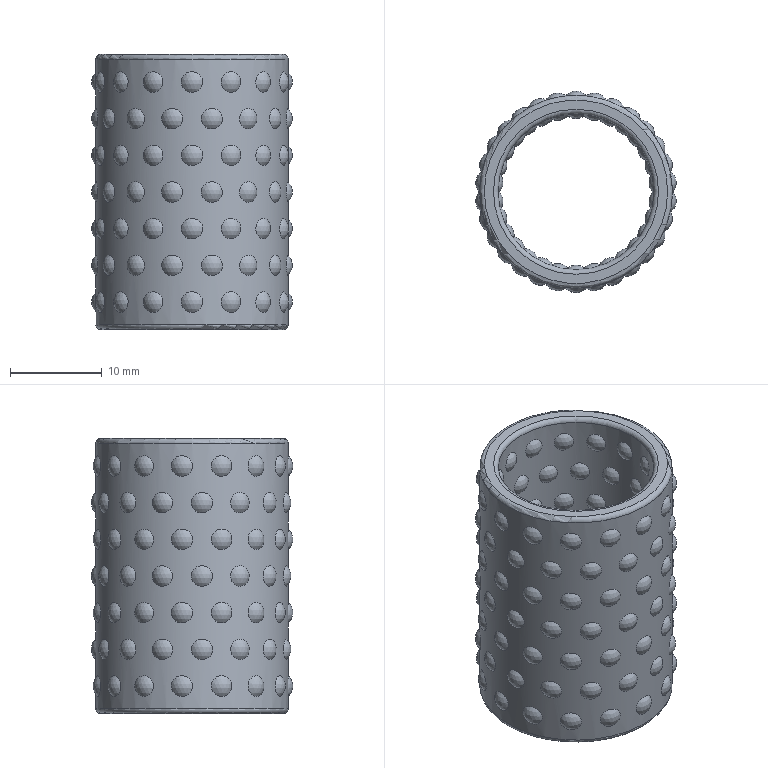Part | STEP file | 200 mesh_id1802 | 1 solid | 218 faces | box 21.896 x 22 x 30 mm | volume 3781 mm3 | sphere 210 | torus 4 | cylinder 2 | plane 2 | commonest cylinder face diameters 17 x1 21 x1